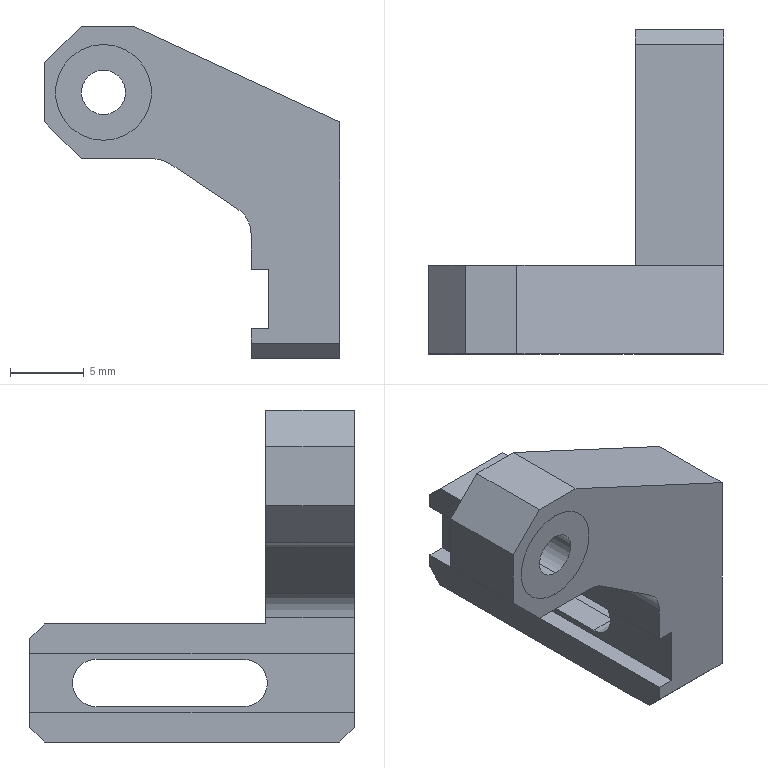Part | SolidWorks | features ICE 10, Chamfer 2, Cut 1, Extrusion 1, Fillet 1 | 2 solids | 43 faces | box 20 x 22 x 22.5 mm | volume 1597 mm3 | plane 29 | cylinder 14 | commonest cylinder face diameters 4 x4 6.5 x4 3 x2 3.2 x2 6 x2
STEP:
#1=CARTESIAN_POINT('',(-6.,-6.,19.5));
#2=VERTEX_POINT('',#1);
#3=CARTESIAN_POINT('',(-6.,-6.,16.5));
#4=VERTEX_POINT('',#3);
#5=CARTESIAN_POINT('',(-6.,-6.,18.));
#6=DIRECTION('',(0.,-1.,0.));
#7=DIRECTION('',(0.,0.,-1.));
#8=AXIS2_PLACEMENT_3D('',#5,#6,#7);
#9=CIRCLE('',#8,1.5);
#10=EDGE_CURVE('',#2,#4,#9,.T.);
#11=ORIENTED_EDGE('',*,*,#10,.F.);
#12=CARTESIAN_POINT('',(-6.,-11.,19.5));
#13=VERTEX_POINT('',#12);
#14=CARTESIAN_POINT('',(-6.,3.192,19.5));
#15=DIRECTION('',(0.,-1.,0.));
#16=VECTOR('',#15,1000.);
#17=LINE('',#14,#16);
#18=EDGE_CURVE('',#2,#13,#17,.T.);
#19=ORIENTED_EDGE('',*,*,#18,.T.);
#20=CARTESIAN_POINT('',(-6.,-11.,16.5));
#21=VERTEX_POINT('',#20);
#22=CARTESIAN_POINT('',(-6.,-11.,18.));
#23=DIRECTION('',(0.,1.,0.));
#24=DIRECTION('',(0.,0.,1.));
#25=AXIS2_PLACEMENT_3D('',#22,#23,#24);
#26=CIRCLE('',#25,1.5);
#27=EDGE_CURVE('',#21,#13,#26,.T.);
#28=ORIENTED_EDGE('',*,*,#27,.F.);
#29=CARTESIAN_POINT('',(-6.,3.192,16.5));
#30=DIRECTION('',(0.,-1.,0.));
#31=VECTOR('',#30,1000.);
#32=LINE('',#29,#31);
#33=EDGE_CURVE('',#4,#21,#32,.T.);
#34=ORIENTED_EDGE('',*,*,#33,.F.);
#35=EDGE_LOOP('',(#11,#19,#28,#34));
#36=FACE_OUTER_BOUND('',#35,.T.);
#37=CARTESIAN_POINT('',(-6.,3.192,18.));
#38=DIRECTION('',(0.,-1.,0.));
#39=DIRECTION('',(0.,0.,-1.));
#40=AXIS2_PLACEMENT_3D('',#37,#38,#39);
#41=CYLINDRICAL_SURFACE('',#40,1.5);
#42=ADVANCED_FACE('',(#36),#41,.F.);
#43=CARTESIAN_POINT('',(-6.,-6.,14.75));
#44=VERTEX_POINT('',#43);
#45=CARTESIAN_POINT('',(-6.,-6.,21.25));
#46=VERTEX_POINT('',#45);
#47=CARTESIAN_POINT('',(-6.,-6.,18.));
#48=DIRECTION('',(0.,-1.,0.));
#49=DIRECTION('',(0.,0.,-1.));
#50=AXIS2_PLACEMENT_3D('',#47,#48,#49);
#51=CIRCLE('',#50,3.25);
#52=EDGE_CURVE('',#44,#46,#51,.T.);
#53=ORIENTED_EDGE('',*,*,#52,.T.);
#54=CARTESIAN_POINT('',(-6.,-11.,21.25));
#55=VERTEX_POINT('',#54);
#56=CARTESIAN_POINT('',(-6.,3.192,21.25));
#57=DIRECTION('',(0.,-1.,0.));
#58=VECTOR('',#57,1000.);
#59=LINE('',#56,#58);
#60=EDGE_CURVE('',#46,#55,#59,.T.);
#61=ORIENTED_EDGE('',*,*,#60,.T.);
#62=CARTESIAN_POINT('',(-6.,-11.,14.75));
#63=VERTEX_POINT('',#62);
#64=CARTESIAN_POINT('',(-6.,-11.,18.));
#65=DIRECTION('',(0.,1.,0.));
#66=DIRECTION('',(0.,0.,1.));
#67=AXIS2_PLACEMENT_3D('',#64,#65,#66);
#68=CIRCLE('',#67,3.25);
#69=EDGE_CURVE('',#55,#63,#68,.T.);
#70=ORIENTED_EDGE('',*,*,#69,.T.);
#71=CARTESIAN_POINT('',(-6.,3.192,14.75));
#72=DIRECTION('',(0.,-1.,0.));
#73=VECTOR('',#72,1000.);
#74=LINE('',#71,#73);
#75=EDGE_CURVE('',#44,#63,#74,.T.);
#76=ORIENTED_EDGE('',*,*,#75,.F.);
#77=EDGE_LOOP('',(#53,#61,#70,#76));
#78=FACE_OUTER_BOUND('',#77,.T.);
#79=CARTESIAN_POINT('',(-6.,3.192,18.));
#80=DIRECTION('',(0.,-1.,0.));
#81=DIRECTION('',(0.,0.,-1.));
#82=AXIS2_PLACEMENT_3D('',#79,#80,#81);
#83=CYLINDRICAL_SURFACE('',#82,3.25);
#84=ADVANCED_FACE('',(#78),#83,.T.);
#85=CARTESIAN_POINT('',(-6.,-11.,18.));
#86=DIRECTION('',(0.,1.,0.));
#87=DIRECTION('',(0.,0.,1.));
#88=AXIS2_PLACEMENT_3D('',#85,#86,#87);
#89=CIRCLE('',#88,3.25);
#90=EDGE_CURVE('',#63,#55,#89,.T.);
#91=ORIENTED_EDGE('',*,*,#90,.F.);
#92=ORIENTED_EDGE('',*,*,#69,.F.);
#93=EDGE_LOOP('',(#91,#92));
#94=FACE_OUTER_BOUND('',#93,.T.);
#95=ORIENTED_EDGE('',*,*,#27,.T.);
#96=CARTESIAN_POINT('',(-6.,-11.,18.));
#97=DIRECTION('',(0.,1.,0.));
#98=DIRECTION('',(0.,0.,1.));
#99=AXIS2_PLACEMENT_3D('',#96,#97,#98);
#100=CIRCLE('',#99,1.5);
#101=EDGE_CURVE('',#13,#21,#100,.T.);
#102=ORIENTED_EDGE('',*,*,#101,.T.);
#103=EDGE_LOOP('',(#95,#102));
#104=FACE_BOUND('',#103,.T.);
#105=CARTESIAN_POINT('',(-6.,-11.,18.));
#106=DIRECTION('',(0.,1.,0.));
#107=DIRECTION('',(0.,0.,1.));
#108=AXIS2_PLACEMENT_3D('',#105,#106,#107);
#109=PLANE('',#108);
#110=ADVANCED_FACE('',(#94,#104),#109,.F.);
#111=ORIENTED_EDGE('',*,*,#60,.F.);
#112=CARTESIAN_POINT('',(-6.,-6.,18.));
#113=DIRECTION('',(0.,-1.,0.));
#114=DIRECTION('',(0.,0.,-1.));
#115=AXIS2_PLACEMENT_3D('',#112,#113,#114);
#116=CIRCLE('',#115,3.25);
#117=EDGE_CURVE('',#46,#44,#116,.T.);
#118=ORIENTED_EDGE('',*,*,#117,.T.);
#119=ORIENTED_EDGE('',*,*,#75,.T.);
#120=ORIENTED_EDGE('',*,*,#90,.T.);
#121=EDGE_LOOP('',(#111,#118,#119,#120));
#122=FACE_OUTER_BOUND('',#121,.T.);
#123=CARTESIAN_POINT('',(-6.,3.192,18.));
#124=DIRECTION('',(0.,-1.,0.));
#125=DIRECTION('',(0.,0.,-1.));
#126=AXIS2_PLACEMENT_3D('',#123,#124,#125);
#127=CYLINDRICAL_SURFACE('',#126,3.25);
#128=ADVANCED_FACE('',(#122),#127,.T.);
#129=ORIENTED_EDGE('',*,*,#18,.F.);
#130=CARTESIAN_POINT('',(-6.,-6.,18.));
#131=DIRECTION('',(0.,-1.,0.));
#132=DIRECTION('',(0.,0.,-1.));
#133=AXIS2_PLACEMENT_3D('',#130,#131,#132);
#134=CIRCLE('',#133,1.5);
#135=EDGE_CURVE('',#4,#2,#134,.T.);
#136=ORIENTED_EDGE('',*,*,#135,.F.);
#137=ORIENTED_EDGE('',*,*,#33,.T.);
#138=ORIENTED_EDGE('',*,*,#101,.F.);
#139=EDGE_LOOP('',(#129,#136,#137,#138));
#140=FACE_OUTER_BOUND('',#139,.T.);
#141=CARTESIAN_POINT('',(-6.,3.192,18.));
#142=DIRECTION('',(0.,-1.,0.));
#143=DIRECTION('',(0.,0.,-1.));
#144=AXIS2_PLACEMENT_3D('',#141,#142,#143);
#145=CYLINDRICAL_SURFACE('',#144,1.5);
#146=ADVANCED_FACE('',(#140),#145,.F.);
#147=ORIENTED_EDGE('',*,*,#52,.F.);
#148=ORIENTED_EDGE('',*,*,#117,.F.);
#149=EDGE_LOOP('',(#147,#148));
#150=FACE_OUTER_BOUND('',#149,.T.);
#151=ORIENTED_EDGE('',*,*,#135,.T.);
#152=ORIENTED_EDGE('',*,*,#10,.T.);
#153=EDGE_LOOP('',(#151,#152));
#154=FACE_BOUND('',#153,.T.);
#155=CARTESIAN_POINT('',(-10.,-6.,22.5));
#156=DIRECTION('',(0.,-1.,0.));
#157=DIRECTION('',(0.,0.,-1.));
#158=AXIS2_PLACEMENT_3D('',#155,#156,#157);
#159=PLANE('',#158);
#160=ADVANCED_FACE('',(#150,#154),#159,.F.);
#161=CLOSED_SHELL('',(#42,#84,#110,#128,#146,#160));
#162=MANIFOLD_SOLID_BREP('',#161);
#163=CARTESIAN_POINT('',(-6.,-6.,16.));
#164=VERTEX_POINT('',#163);
#165=CARTESIAN_POINT('',(-6.,-6.,20.));
#166=VERTEX_POINT('',#165);
#167=CARTESIAN_POINT('',(-6.,-6.,18.));
#168=DIRECTION('',(0.,1.,0.));
#169=DIRECTION('',(0.,0.,1.));
#170=AXIS2_PLACEMENT_3D('',#167,#168,#169);
#171=CIRCLE('',#170,2.);
#172=EDGE_CURVE('',#164,#166,#171,.T.);
#173=ORIENTED_EDGE('',*,*,#172,.F.);
#174=CARTESIAN_POINT('',(-6.,-5.,16.));
#175=VERTEX_POINT('',#174);
#176=CARTESIAN_POINT('',(-6.,-6.,16.));
#177=DIRECTION('',(0.,1.,0.));
#178=VECTOR('',#177,1000.);
#179=LINE('',#176,#178);
#180=EDGE_CURVE('',#164,#175,#179,.T.);
#181=ORIENTED_EDGE('',*,*,#180,.T.);
#182=CARTESIAN_POINT('',(-6.,-5.,20.));
#183=VERTEX_POINT('',#182);
#184=CARTESIAN_POINT('',(-6.,-5.,18.));
#185=DIRECTION('',(0.,1.,0.));
#186=DIRECTION('',(0.,0.,1.));
#187=AXIS2_PLACEMENT_3D('',#184,#185,#186);
#188=CIRCLE('',#187,2.);
#189=EDGE_CURVE('',#175,#183,#188,.T.);
#190=ORIENTED_EDGE('',*,*,#189,.T.);
#191=CARTESIAN_POINT('',(-6.,-6.,20.));
#192=DIRECTION('',(0.,1.,0.));
#193=VECTOR('',#192,1000.);
#194=LINE('',#191,#193);
#195=EDGE_CURVE('',#166,#183,#194,.T.);
#196=ORIENTED_EDGE('',*,*,#195,.F.);
#197=EDGE_LOOP('',(#173,#181,#190,#196));
#198=FACE_OUTER_BOUND('',#197,.T.);
#199=CARTESIAN_POINT('',(-6.,-6.,18.));
#200=DIRECTION('',(0.,1.,0.));
#201=DIRECTION('',(0.,0.,1.));
#202=AXIS2_PLACEMENT_3D('',#199,#200,#201);
#203=CYLINDRICAL_SURFACE('',#202,2.);
#204=ADVANCED_FACE('',(#198),#203,.F.);
#205=CARTESIAN_POINT('',(-6.,-6.,21.25));
#206=VERTEX_POINT('',#205);
#207=CARTESIAN_POINT('',(-6.,-6.,14.75));
#208=VERTEX_POINT('',#207);
#209=CARTESIAN_POINT('',(-6.,-6.,18.));
#210=DIRECTION('',(0.,-1.,0.));
#211=DIRECTION('',(0.,0.,-1.));
#212=AXIS2_PLACEMENT_3D('',#209,#210,#211);
#213=CIRCLE('',#212,3.25);
#214=EDGE_CURVE('',#206,#208,#213,.T.);
#215=ORIENTED_EDGE('',*,*,#214,.F.);
#216=CARTESIAN_POINT('',(-6.,-11.,21.25));
#217=VERTEX_POINT('',#216);
#218=CARTESIAN_POINT('',(-6.,4.192,21.25));
#219=DIRECTION('',(0.,-1.,0.));
#220=VECTOR('',#219,1000.);
#221=LINE('',#218,#220);
#222=EDGE_CURVE('',#206,#217,#221,.T.);
#223=ORIENTED_EDGE('',*,*,#222,.T.);
#224=CARTESIAN_POINT('',(-6.,-11.,14.75));
#225=VERTEX_POINT('',#224);
#226=CARTESIAN_POINT('',(-6.,-11.,18.));
#227=DIRECTION('',(0.,1.,0.));
#228=DIRECTION('',(0.,0.,1.));
#229=AXIS2_PLACEMENT_3D('',#226,#227,#228);
#230=CIRCLE('',#229,3.25);
#231=EDGE_CURVE('',#225,#217,#230,.T.);
#232=ORIENTED_EDGE('',*,*,#231,.F.);
#233=CARTESIAN_POINT('',(-6.,4.192,14.75));
#234=DIRECTION('',(0.,-1.,0.));
#235=VECTOR('',#234,1000.);
#236=LINE('',#233,#235);
#237=EDGE_CURVE('',#208,#225,#236,.T.);
#238=ORIENTED_EDGE('',*,*,#237,.F.);
#239=EDGE_LOOP('',(#215,#223,#232,#238));
#240=FACE_OUTER_BOUND('',#239,.T.);
#241=CARTESIAN_POINT('',(-6.,4.192,18.));
#242=DIRECTION('',(0.,-1.,0.));
#243=DIRECTION('',(0.,0.,-1.));
#244=AXIS2_PLACEMENT_3D('',#241,#242,#243);
#245=CYLINDRICAL_SURFACE('',#244,3.25);
#246=ADVANCED_FACE('',(#240),#245,.F.);
#247=CARTESIAN_POINT('',(7.,-3.5,2.4));
#248=VERTEX_POINT('',#247);
#249=CARTESIAN_POINT('',(7.,-3.5,5.6));
#250=VERTEX_POINT('',#249);
#251=CARTESIAN_POINT('',(7.,-3.5,4.));
#252=DIRECTION('',(-1.,0.,0.));
#253=DIRECTION('',(0.,0.,-1.));
#254=AXIS2_PLACEMENT_3D('',#251,#252,#253);
#255=CIRCLE('',#254,1.6);
#256=EDGE_CURVE('',#248,#250,#255,.T.);
#257=ORIENTED_EDGE('',*,*,#256,.F.);
#258=CARTESIAN_POINT('',(5.2,-3.5,2.4));
#259=VERTEX_POINT('',#258);
#260=CARTESIAN_POINT('',(-10.,-3.5,2.4));
#261=DIRECTION('',(1.,0.,0.));
#262=VECTOR('',#261,1000.);
#263=LINE('',#260,#262);
#264=EDGE_CURVE('',#259,#248,#263,.T.);
#265=ORIENTED_EDGE('',*,*,#264,.F.);
#266=CARTESIAN_POINT('',(5.2,-3.5,5.6));
#267=VERTEX_POINT('',#266);
#268=CARTESIAN_POINT('',(5.2,-3.5,4.));
#269=DIRECTION('',(-1.,0.,0.));
#270=DIRECTION('',(0.,0.,1.));
#271=AXIS2_PLACEMENT_3D('',#268,#269,#270);
#272=CIRCLE('',#271,1.6);
#273=EDGE_CURVE('',#259,#267,#272,.T.);
#274=ORIENTED_EDGE('',*,*,#273,.T.);
#275=CARTESIAN_POINT('',(-10.,-3.5,5.6));
#276=DIRECTION('',(1.,0.,0.));
#277=VECTOR('',#276,1000.);
#278=LINE('',#275,#277);
#279=EDGE_CURVE('',#267,#250,#278,.T.);
#280=ORIENTED_EDGE('',*,*,#279,.T.);
#281=EDGE_LOOP('',(#257,#265,#274,#280));
#282=FACE_OUTER_BOUND('',#281,.T.);
#283=CARTESIAN_POINT('',(-10.,-3.5,4.));
#284=DIRECTION('',(1.,0.,0.));
#285=DIRECTION('',(0.,0.,-1.));
#286=AXIS2_PLACEMENT_3D('',#283,#284,#285);
#287=CYLINDRICAL_SURFACE('',#286,1.6);
#288=ADVANCED_FACE('',(#282),#287,.F.);
#289=CARTESIAN_POINT('',(7.,6.5,5.6));
#290=VERTEX_POINT('',#289);
#291=CARTESIAN_POINT('',(7.,-3.5,5.6));
#292=DIRECTION('',(0.,1.,0.));
#293=VECTOR('',#292,1000.);
#294=LINE('',#291,#293);
#295=EDGE_CURVE('',#250,#290,#294,.T.);
#296=ORIENTED_EDGE('',*,*,#295,.F.);
#297=ORIENTED_EDGE('',*,*,#279,.F.);
#298=CARTESIAN_POINT('',(5.2,6.5,5.6));
#299=VERTEX_POINT('',#298);
#300=CARTESIAN_POINT('',(5.2,0.,5.6));
#301=DIRECTION('',(0.,1.,0.));
#302=VECTOR('',#301,1000.);
#303=LINE('',#300,#302);
#304=EDGE_CURVE('',#267,#299,#303,.T.);
#305=ORIENTED_EDGE('',*,*,#304,.T.);
#306=CARTESIAN_POINT('',(-10.,6.5,5.6));
#307=DIRECTION('',(1.,0.,0.));
#308=VECTOR('',#307,1000.);
#309=LINE('',#306,#308);
#310=EDGE_CURVE('',#299,#290,#309,.T.);
#311=ORIENTED_EDGE('',*,*,#310,.T.);
#312=EDGE_LOOP('',(#296,#297,#305,#311));
#313=FACE_OUTER_BOUND('',#312,.T.);
#314=CARTESIAN_POINT('',(-10.,-3.5,5.6));
#315=DIRECTION('',(0.,0.,1.));
#316=DIRECTION('',(1.,0.,0.));
#317=AXIS2_PLACEMENT_3D('',#314,#315,#316);
#318=PLANE('',#317);
#319=ADVANCED_FACE('',(#313),#318,.F.);
#320=CARTESIAN_POINT('',(7.,6.5,2.4));
#321=VERTEX_POINT('',#320);
#322=CARTESIAN_POINT('',(7.,6.5,4.));
#323=DIRECTION('',(-1.,0.,0.));
#324=DIRECTION('',(0.,0.,-1.));
#325=AXIS2_PLACEMENT_3D('',#322,#323,#324);
#326=CIRCLE('',#325,1.6);
#327=EDGE_CURVE('',#290,#321,#326,.T.);
#328=ORIENTED_EDGE('',*,*,#327,.F.);
#329=ORIENTED_EDGE('',*,*,#310,.F.);
#330=CARTESIAN_POINT('',(5.2,6.5,2.4));
#331=VERTEX_POINT('',#330);
#332=CARTESIAN_POINT('',(5.2,6.5,4.));
#333=DIRECTION('',(-1.,0.,0.));
#334=DIRECTION('',(0.,0.,1.));
#335=AXIS2_PLACEMENT_3D('',#332,#333,#334);
#336=CIRCLE('',#335,1.6);
#337=EDGE_CURVE('',#299,#331,#336,.T.);
#338=ORIENTED_EDGE('',*,*,#337,.T.);
#339=CARTESIAN_POINT('',(-10.,6.5,2.4));
#340=DIRECTION('',(1.,0.,0.));
#341=VECTOR('',#340,1000.);
#342=LINE('',#339,#341);
#343=EDGE_CURVE('',#331,#321,#342,.T.);
#344=ORIENTED_EDGE('',*,*,#343,.T.);
#345=EDGE_LOOP('',(#328,#329,#338,#344));
#346=FACE_OUTER_BOUND('',#345,.T.);
#347=CARTESIAN_POINT('',(-10.,6.5,4.));
#348=DIRECTION('',(1.,0.,0.));
#349=DIRECTION('',(0.,0.,-1.));
#350=AXIS2_PLACEMENT_3D('',#347,#348,#349);
#351=CYLINDRICAL_SURFACE('',#350,1.6);
#352=ADVANCED_FACE('',(#346),#351,.F.);
#353=CARTESIAN_POINT('',(7.,-3.5,2.4));
#354=DIRECTION('',(0.,-1.,0.));
#355=VECTOR('',#354,1000.);
#356=LINE('',#353,#355);
#357=EDGE_CURVE('',#321,#248,#356,.T.);
#358=ORIENTED_EDGE('',*,*,#357,.F.);
#359=ORIENTED_EDGE('',*,*,#343,.F.);
#360=CARTESIAN_POINT('',(5.2,0.,2.4));
#361=DIRECTION('',(0.,-1.,0.));
#362=VECTOR('',#361,1000.);
#363=LINE('',#360,#362);
#364=EDGE_CURVE('',#331,#259,#363,.T.);
#365=ORIENTED_EDGE('',*,*,#364,.T.);
#366=ORIENTED_EDGE('',*,*,#264,.T.);
#367=EDGE_LOOP('',(#358,#359,#365,#366));
#368=FACE_OUTER_BOUND('',#367,.T.);
#369=CARTESIAN_POINT('',(-10.,-3.5,2.4));
#370=DIRECTION('',(0.,0.,-1.));
#371=DIRECTION('',(-1.,0.,0.));
#372=AXIS2_PLACEMENT_3D('',#369,#370,#371);
#373=PLANE('',#372);
#374=ADVANCED_FACE('',(#368),#373,.F.);
#375=CARTESIAN_POINT('',(4.,-11.,6.));
#376=VERTEX_POINT('',#375);
#377=CARTESIAN_POINT('',(4.,-11.,8.43));
#378=VERTEX_POINT('',#377);
#379=CARTESIAN_POINT('',(4.,-11.,0.));
#380=DIRECTION('',(0.,0.,1.));
#381=VECTOR('',#380,1000.);
#382=LINE('',#379,#381);
#383=EDGE_CURVE('',#376,#378,#382,.T.);
#384=ORIENTED_EDGE('',*,*,#383,.T.);
#385=CARTESIAN_POINT('',(4.,-5.,8.43));
#386=VERTEX_POINT('',#385);
#387=CARTESIAN_POINT('',(4.,11.,8.43));
#388=DIRECTION('',(0.,1.,0.));
#389=VECTOR('',#388,1000.);
#390=LINE('',#387,#389);
#391=EDGE_CURVE('',#378,#386,#390,.T.);
#392=ORIENTED_EDGE('',*,*,#391,.T.);
#393=CARTESIAN_POINT('',(4.,-5.,8.));
#394=VERTEX_POINT('',#393);
#395=CARTESIAN_POINT('',(4.,-5.,22.5));
#396=DIRECTION('',(0.,0.,1.));
#397=VECTOR('',#396,1000.);
#398=LINE('',#395,#397);
#399=EDGE_CURVE('',#394,#386,#398,.T.);
#400=ORIENTED_EDGE('',*,*,#399,.F.);
#401=CARTESIAN_POINT('',(4.,10.,8.));
#402=VERTEX_POINT('',#401);
#403=CARTESIAN_POINT('',(4.,0.,8.));
#404=DIRECTION('',(0.,-1.,0.));
#405=VECTOR('',#404,1000.);
#406=LINE('',#403,#405);
#407=EDGE_CURVE('',#402,#394,#406,.T.);
#408=ORIENTED_EDGE('',*,*,#407,.F.);
#409=CARTESIAN_POINT('',(4.,11.,7.));
#410=VERTEX_POINT('',#409);
#411=CARTESIAN_POINT('',(4.,10.,8.));
#412=DIRECTION('',(0.,0.7071,-0.7071));
#413=VECTOR('',#412,1000.);
#414=LINE('',#411,#413);
#415=EDGE_CURVE('',#402,#410,#414,.T.);
#416=ORIENTED_EDGE('',*,*,#415,.T.);
#417=CARTESIAN_POINT('',(4.,11.,6.));
#418=VERTEX_POINT('',#417);
#419=CARTESIAN_POINT('',(4.,11.,8.));
#420=DIRECTION('',(0.,0.,1.));
#421=VECTOR('',#420,1000.);
#422=LINE('',#419,#421);
#423=EDGE_CURVE('',#418,#410,#422,.T.);
#424=ORIENTED_EDGE('',*,*,#423,.F.);
#425=CARTESIAN_POINT('',(4.,-11.,6.));
#426=DIRECTION('',(0.,1.,0.));
#427=VECTOR('',#426,1000.);
#428=LINE('',#425,#427);
#429=EDGE_CURVE('',#376,#418,#428,.T.);
#430=ORIENTED_EDGE('',*,*,#429,.F.);
#431=EDGE_LOOP('',(#384,#392,#400,#408,#416,#424,#430));
#432=FACE_OUTER_BOUND('',#431,.T.);
#433=CARTESIAN_POINT('',(4.,11.,0.));
#434=DIRECTION('',(1.,0.,0.));
#435=DIRECTION('',(0.,0.,-1.));
#436=AXIS2_PLACEMENT_3D('',#433,#434,#435);
#437=PLANE('',#436);
#438=ADVANCED_FACE('',(#432),#437,.F.);
#439=CARTESIAN_POINT('',(4.,-11.,1.));
#440=VERTEX_POINT('',#439);
#441=CARTESIAN_POINT('',(4.,-11.,2.));
#442=VERTEX_POINT('',#441);
#443=CARTESIAN_POINT('',(4.,-11.,0.));
#444=DIRECTION('',(0.,0.,1.));
#445=VECTOR('',#444,1000.);
#446=LINE('',#443,#445);
#447=EDGE_CURVE('',#440,#442,#446,.T.);
#448=ORIENTED_EDGE('',*,*,#447,.F.);
#449=CARTESIAN_POINT('',(10.,-11.,1.));
#450=VERTEX_POINT('',#449);
#451=CARTESIAN_POINT('',(10.,-11.,1.));
#452=DIRECTION('',(1.,0.,0.));
#453=VECTOR('',#452,1000.);
#454=LINE('',#451,#453);
#455=EDGE_CURVE('',#440,#450,#454,.T.);
#456=ORIENTED_EDGE('',*,*,#455,.T.);
#457=CARTESIAN_POINT('',(10.,-11.,16.));
#458=VERTEX_POINT('',#457);
#459=CARTESIAN_POINT('',(10.,-11.,8.));
#460=DIRECTION('',(0.,0.,-1.));
#461=VECTOR('',#460,1000.);
#462=LINE('',#459,#461);
#463=EDGE_CURVE('',#458,#450,#462,.T.);
#464=ORIENTED_EDGE('',*,*,#463,.F.);
#465=CARTESIAN_POINT('',(-4.,-11.,22.5));
#466=VERTEX_POINT('',#465);
#467=CARTESIAN_POINT('',(-4.,-11.,22.5));
#468=DIRECTION('',(0.907,0.,-0.4211));
#469=VECTOR('',#468,1000.);
#470=LINE('',#467,#469);
#471=EDGE_CURVE('',#466,#458,#470,.T.);
#472=ORIENTED_EDGE('',*,*,#471,.F.);
#473=CARTESIAN_POINT('',(-7.5,-11.,22.5));
#474=VERTEX_POINT('',#473);
#475=CARTESIAN_POINT('',(-10.,-11.,22.5));
#476=DIRECTION('',(1.,0.,0.));
#477=VECTOR('',#476,1000.);
#478=LINE('',#475,#477);
#479=EDGE_CURVE('',#474,#466,#478,.T.);
#480=ORIENTED_EDGE('',*,*,#479,.F.);
#481=CARTESIAN_POINT('',(-10.,-11.,20.));
#482=VERTEX_POINT('',#481);
#483=CARTESIAN_POINT('',(-7.5,-11.,22.5));
#484=DIRECTION('',(-0.7071,0.,-0.7071));
#485=VECTOR('',#484,1000.);
#486=LINE('',#483,#485);
#487=EDGE_CURVE('',#474,#482,#486,.T.);
#488=ORIENTED_EDGE('',*,*,#487,.T.);
#489=CARTESIAN_POINT('',(-10.,-11.,16.));
#490=VERTEX_POINT('',#489);
#491=CARTESIAN_POINT('',(-10.,-11.,8.));
#492=DIRECTION('',(0.,0.,-1.));
#493=VECTOR('',#492,1000.);
#494=LINE('',#491,#493);
#495=EDGE_CURVE('',#482,#490,#494,.T.);
#496=ORIENTED_EDGE('',*,*,#495,.T.);
#497=CARTESIAN_POINT('',(-7.5,-11.,13.5));
#498=VERTEX_POINT('',#497);
#499=CARTESIAN_POINT('',(-10.,-11.,16.));
#500=DIRECTION('',(0.7071,0.,-0.7071));
#501=VECTOR('',#500,1000.);
#502=LINE('',#499,#501);
#503=EDGE_CURVE('',#490,#498,#502,.T.);
#504=ORIENTED_EDGE('',*,*,#503,.T.);
#505=CARTESIAN_POINT('',(-2.606,-11.,13.5));
#506=VERTEX_POINT('',#505);
#507=CARTESIAN_POINT('',(4.,-11.,13.5));
#508=DIRECTION('',(-1.,0.,0.));
#509=VECTOR('',#508,1000.);
#510=LINE('',#507,#509);
#511=EDGE_CURVE('',#506,#498,#510,.T.);
#512=ORIENTED_EDGE('',*,*,#511,.F.);
#513=CARTESIAN_POINT('',(-1.496,-11.,13.164));
#514=VERTEX_POINT('',#513);
#515=CARTESIAN_POINT('',(-2.606,-11.,11.5));
#516=DIRECTION('',(0.,1.,0.));
#517=DIRECTION('',(0.,0.,1.));
#518=AXIS2_PLACEMENT_3D('',#515,#516,#517);
#519=CIRCLE('',#518,2.);
#520=EDGE_CURVE('',#506,#514,#519,.T.);
#521=ORIENTED_EDGE('',*,*,#520,.T.);
#522=CARTESIAN_POINT('',(3.109,-11.,10.094));
#523=VERTEX_POINT('',#522);
#524=CARTESIAN_POINT('',(-2.,-11.,13.5));
#525=DIRECTION('',(0.8321,0.,-0.5547));
#526=VECTOR('',#525,1000.);
#527=LINE('',#524,#526);
#528=EDGE_CURVE('',#514,#523,#527,.T.);
#529=ORIENTED_EDGE('',*,*,#528,.T.);
#530=CARTESIAN_POINT('',(2.,-11.,8.43));
#531=DIRECTION('',(0.,1.,0.));
#532=DIRECTION('',(0.,0.,1.));
#533=AXIS2_PLACEMENT_3D('',#530,#531,#532);
#534=CIRCLE('',#533,2.);
#535=EDGE_CURVE('',#523,#378,#534,.T.);
#536=ORIENTED_EDGE('',*,*,#535,.T.);
#537=ORIENTED_EDGE('',*,*,#383,.F.);
#538=CARTESIAN_POINT('',(5.2,-11.,6.));
#539=VERTEX_POINT('',#538);
#540=CARTESIAN_POINT('',(5.2,-11.,6.));
#541=DIRECTION('',(-1.,0.,0.));
#542=VECTOR('',#541,1000.);
#543=LINE('',#540,#542);
#544=EDGE_CURVE('',#539,#376,#543,.T.);
#545=ORIENTED_EDGE('',*,*,#544,.F.);
#546=CARTESIAN_POINT('',(5.2,-11.,2.));
#547=VERTEX_POINT('',#546);
#548=CARTESIAN_POINT('',(5.2,-11.,6.));
#549=DIRECTION('',(0.,0.,1.));
#550=VECTOR('',#549,1000.);
#551=LINE('',#548,#550);
#552=EDGE_CURVE('',#547,#539,#551,.T.);
#553=ORIENTED_EDGE('',*,*,#552,.F.);
#554=CARTESIAN_POINT('',(5.2,-11.,2.));
#555=DIRECTION('',(-1.,0.,0.));
#556=VECTOR('',#555,1000.);
#557=LINE('',#554,#556);
#558=EDGE_CURVE('',#547,#442,#557,.T.);
#559=ORIENTED_EDGE('',*,*,#558,.T.);
#560=EDGE_LOOP('',(#448,#456,#464,#472,#480,#488,#496,#504,#512,#521,#529,#536,#537,#545,#553,#559));
#561=FACE_OUTER_BOUND('',#560,.T.);
#562=ORIENTED_EDGE('',*,*,#231,.T.);
#563=CARTESIAN_POINT('',(-6.,-11.,18.));
#564=DIRECTION('',(0.,1.,0.));
#565=DIRECTION('',(0.,0.,1.));
#566=AXIS2_PLACEMENT_3D('',#563,#564,#565);
#567=CIRCLE('',#566,3.25);
#568=EDGE_CURVE('',#217,#225,#567,.T.);
#569=ORIENTED_EDGE('',*,*,#568,.T.);
#570=EDGE_LOOP('',(#562,#569));
#571=FACE_BOUND('',#570,.T.);
#572=CARTESIAN_POINT('',(-10.,-11.,8.));
#573=DIRECTION('',(0.,1.,0.));
#574=DIRECTION('',(0.,0.,1.));
#575=AXIS2_PLACEMENT_3D('',#572,#573,#574);
#576=PLANE('',#575);
#577=ADVANCED_FACE('',(#561,#571),#576,.F.);
#578=CARTESIAN_POINT('',(10.,-5.,8.));
#579=VERTEX_POINT('',#578);
#580=CARTESIAN_POINT('',(10.,10.,8.));
#581=VERTEX_POINT('',#580);
#582=CARTESIAN_POINT('',(10.,-11.,8.));
#583=DIRECTION('',(0.,1.,0.));
#584=VECTOR('',#583,1000.);
#585=LINE('',#582,#584);
#586=EDGE_CURVE('',#579,#581,#585,.T.);
#587=ORIENTED_EDGE('',*,*,#586,.T.);
#588=CARTESIAN_POINT('',(0.,10.,8.));
#589=DIRECTION('',(-1.,0.,0.));
#590=VECTOR('',#589,1000.);
#591=LINE('',#588,#590);
#592=EDGE_CURVE('',#581,#402,#591,.T.);
#593=ORIENTED_EDGE('',*,*,#592,.T.);
#594=ORIENTED_EDGE('',*,*,#407,.T.);
#595=CARTESIAN_POINT('',(-10.,-5.,8.));
#596=DIRECTION('',(-1.,0.,0.));
#597=VECTOR('',#596,1000.);
#598=LINE('',#595,#597);
#599=EDGE_CURVE('',#579,#394,#598,.T.);
#600=ORIENTED_EDGE('',*,*,#599,.F.);
#601=EDGE_LOOP('',(#587,#593,#594,#600));
#602=FACE_OUTER_BOUND('',#601,.T.);
#603=CARTESIAN_POINT('',(0.,0.,8.));
#604=DIRECTION('',(0.,0.,-1.));
#605=DIRECTION('',(-1.,0.,0.));
#606=AXIS2_PLACEMENT_3D('',#603,#604,#605);
#607=PLANE('',#606);
#608=ADVANCED_FACE('',(#602),#607,.F.);
#609=CARTESIAN_POINT('',(10.,-3.5,1.));
#610=VERTEX_POINT('',#609);
#611=CARTESIAN_POINT('',(10.,6.5,1.));
#612=VERTEX_POINT('',#611);
#613=CARTESIAN_POINT('',(10.,-3.5,1.));
#614=DIRECTION('',(0.,1.,0.));
#615=VECTOR('',#614,1000.);
#616=LINE('',#613,#615);
#617=EDGE_CURVE('',#610,#612,#616,.T.);
#618=ORIENTED_EDGE('',*,*,#617,.F.);
#619=CARTESIAN_POINT('',(10.,-3.5,7.));
#620=VERTEX_POINT('',#619);
#621=CARTESIAN_POINT('',(10.,-3.5,4.));
#622=DIRECTION('',(1.,0.,0.));
#623=DIRECTION('',(0.,0.,-1.));
#624=AXIS2_PLACEMENT_3D('',#621,#622,#623);
#625=CIRCLE('',#624,3.);
#626=EDGE_CURVE('',#620,#610,#625,.T.);
#627=ORIENTED_EDGE('',*,*,#626,.F.);
#628=CARTESIAN_POINT('',(10.,6.5,7.));
#629=VERTEX_POINT('',#628);
#630=CARTESIAN_POINT('',(10.,-3.5,7.));
#631=DIRECTION('',(0.,-1.,0.));
#632=VECTOR('',#631,1000.);
#633=LINE('',#630,#632);
#634=EDGE_CURVE('',#629,#620,#633,.T.);
#635=ORIENTED_EDGE('',*,*,#634,.F.);
#636=CARTESIAN_POINT('',(10.,6.5,4.));
#637=DIRECTION('',(1.,0.,0.));
#638=DIRECTION('',(0.,0.,-1.));
#639=AXIS2_PLACEMENT_3D('',#636,#637,#638);
#640=CIRCLE('',#639,3.);
#641=EDGE_CURVE('',#612,#629,#640,.T.);
#642=ORIENTED_EDGE('',*,*,#641,.F.);
#643=EDGE_LOOP('',(#618,#627,#635,#642));
#644=FACE_BOUND('',#643,.T.);
#645=ORIENTED_EDGE('',*,*,#463,.T.);
#646=CARTESIAN_POINT('',(10.,-10.,0.));
#647=VERTEX_POINT('',#646);
#648=CARTESIAN_POINT('',(10.,-11.,1.));
#649=DIRECTION('',(0.,0.7071,-0.7071));
#650=VECTOR('',#649,1000.);
#651=LINE('',#648,#650);
#652=EDGE_CURVE('',#450,#647,#651,.T.);
#653=ORIENTED_EDGE('',*,*,#652,.T.);
#654=CARTESIAN_POINT('',(10.,10.,0.));
#655=VERTEX_POINT('',#654);
#656=CARTESIAN_POINT('',(10.,-11.,0.));
#657=DIRECTION('',(0.,1.,0.));
#658=VECTOR('',#657,1000.);
#659=LINE('',#656,#658);
#660=EDGE_CURVE('',#647,#655,#659,.T.);
#661=ORIENTED_EDGE('',*,*,#660,.T.);
#662=CARTESIAN_POINT('',(10.,11.,1.));
#663=VERTEX_POINT('',#662);
#664=CARTESIAN_POINT('',(10.,11.,1.));
#665=DIRECTION('',(0.,0.7071,0.7071));
#666=VECTOR('',#665,1000.);
#667=LINE('',#664,#666);
#668=EDGE_CURVE('',#655,#663,#667,.T.);
#669=ORIENTED_EDGE('',*,*,#668,.T.);
#670=CARTESIAN_POINT('',(10.,11.,7.));
#671=VERTEX_POINT('',#670);
#672=CARTESIAN_POINT('',(10.,11.,8.));
#673=DIRECTION('',(0.,0.,-1.));
#674=VECTOR('',#673,1000.);
#675=LINE('',#672,#674);
#676=EDGE_CURVE('',#671,#663,#675,.T.);
#677=ORIENTED_EDGE('',*,*,#676,.F.);
#678=CARTESIAN_POINT('',(10.,10.,8.));
#679=DIRECTION('',(0.,-0.7071,0.7071));
#680=VECTOR('',#679,1000.);
#681=LINE('',#678,#680);
#682=EDGE_CURVE('',#671,#581,#681,.T.);
#683=ORIENTED_EDGE('',*,*,#682,.T.);
#684=ORIENTED_EDGE('',*,*,#586,.F.);
#685=CARTESIAN_POINT('',(10.,-5.,16.));
#686=VERTEX_POINT('',#685);
#687=CARTESIAN_POINT('',(10.,-5.,22.5));
#688=DIRECTION('',(0.,0.,-1.));
#689=VECTOR('',#688,1000.);
#690=LINE('',#687,#689);
#691=EDGE_CURVE('',#686,#579,#690,.T.);
#692=ORIENTED_EDGE('',*,*,#691,.F.);
#693=CARTESIAN_POINT('',(10.,11.,16.));
#694=DIRECTION('',(0.,-1.,0.));
#695=VECTOR('',#694,1000.);
#696=LINE('',#693,#695);
#697=EDGE_CURVE('',#686,#458,#696,.T.);
#698=ORIENTED_EDGE('',*,*,#697,.T.);
#699=EDGE_LOOP('',(#645,#653,#661,#669,#677,#683,#684,#692,#698));
#700=FACE_OUTER_BOUND('',#699,.T.);
#701=CARTESIAN_POINT('',(10.,-11.,8.));
#702=DIRECTION('',(-1.,0.,0.));
#703=DIRECTION('',(0.,0.,1.));
#704=AXIS2_PLACEMENT_3D('',#701,#702,#703);
#705=PLANE('',#704);
#706=ADVANCED_FACE('',(#644,#700),#705,.F.);
#707=ORIENTED_EDGE('',*,*,#423,.T.);
#708=CARTESIAN_POINT('',(-10.,11.,7.));
#709=DIRECTION('',(1.,0.,0.));
#710=VECTOR('',#709,1000.);
#711=LINE('',#708,#710);
#712=EDGE_CURVE('',#410,#671,#711,.T.);
#713=ORIENTED_EDGE('',*,*,#712,.T.);
#714=ORIENTED_EDGE('',*,*,#676,.T.);
#715=CARTESIAN_POINT('',(4.,11.,1.));
#716=VERTEX_POINT('',#715);
#717=CARTESIAN_POINT('',(4.,11.,1.));
#718=DIRECTION('',(-1.,0.,0.));
#719=VECTOR('',#718,1000.);
#720=LINE('',#717,#719);
#721=EDGE_CURVE('',#663,#716,#720,.T.);
#722=ORIENTED_EDGE('',*,*,#721,.T.);
#723=CARTESIAN_POINT('',(4.,11.,2.));
#724=VERTEX_POINT('',#723);
#725=CARTESIAN_POINT('',(4.,11.,8.));
#726=DIRECTION('',(0.,0.,1.));
#727=VECTOR('',#726,1000.);
#728=LINE('',#725,#727);
#729=EDGE_CURVE('',#716,#724,#728,.T.);
#730=ORIENTED_EDGE('',*,*,#729,.T.);
#731=CARTESIAN_POINT('',(5.2,11.,2.));
#732=VERTEX_POINT('',#731);
#733=CARTESIAN_POINT('',(5.2,11.,2.));
#734=DIRECTION('',(-1.,0.,0.));
#735=VECTOR('',#734,1000.);
#736=LINE('',#733,#735);
#737=EDGE_CURVE('',#732,#724,#736,.T.);
#738=ORIENTED_EDGE('',*,*,#737,.F.);
#739=CARTESIAN_POINT('',(5.2,11.,6.));
#740=VERTEX_POINT('',#739);
#741=CARTESIAN_POINT('',(5.2,11.,6.));
#742=DIRECTION('',(0.,0.,-1.));
#743=VECTOR('',#742,1000.);
#744=LINE('',#741,#743);
#745=EDGE_CURVE('',#740,#732,#744,.T.);
#746=ORIENTED_EDGE('',*,*,#745,.F.);
#747=CARTESIAN_POINT('',(5.2,11.,6.));
#748=DIRECTION('',(-1.,0.,0.));
#749=VECTOR('',#748,1000.);
#750=LINE('',#747,#749);
#751=EDGE_CURVE('',#740,#418,#750,.T.);
#752=ORIENTED_EDGE('',*,*,#751,.T.);
#753=EDGE_LOOP('',(#707,#713,#714,#722,#730,#738,#746,#752));
#754=FACE_OUTER_BOUND('',#753,.T.);
#755=CARTESIAN_POINT('',(-10.,11.,8.));
#756=DIRECTION('',(0.,-1.,0.));
#757=DIRECTION('',(0.,0.,-1.));
#758=AXIS2_PLACEMENT_3D('',#755,#756,#757);
#759=PLANE('',#758);
#760=ADVANCED_FACE('',(#754),#759,.F.);
#761=ORIENTED_EDGE('',*,*,#495,.F.);
#762=CARTESIAN_POINT('',(-10.,-5.,20.));
#763=VERTEX_POINT('',#762);
#764=CARTESIAN_POINT('',(-10.,-11.,20.));
#765=DIRECTION('',(0.,1.,0.));
#766=VECTOR('',#765,1000.);
#767=LINE('',#764,#766);
#768=EDGE_CURVE('',#482,#763,#767,.T.);
#769=ORIENTED_EDGE('',*,*,#768,.T.);
#770=CARTESIAN_POINT('',(-10.,-5.,16.));
#771=VERTEX_POINT('',#770);
#772=CARTESIAN_POINT('',(-10.,-5.,22.5));
#773=DIRECTION('',(0.,0.,-1.));
#774=VECTOR('',#773,1000.);
#775=LINE('',#772,#774);
#776=EDGE_CURVE('',#763,#771,#775,.T.);
#777=ORIENTED_EDGE('',*,*,#776,.T.);
#778=CARTESIAN_POINT('',(-10.,-11.,16.));
#779=DIRECTION('',(0.,-1.,0.));
#780=VECTOR('',#779,1000.);
#781=LINE('',#778,#780);
#782=EDGE_CURVE('',#771,#490,#781,.T.);
#783=ORIENTED_EDGE('',*,*,#782,.T.);
#784=EDGE_LOOP('',(#761,#769,#777,#783));
#785=FACE_OUTER_BOUND('',#784,.T.);
#786=CARTESIAN_POINT('',(-10.,-11.,8.));
#787=DIRECTION('',(1.,0.,0.));
#788=DIRECTION('',(0.,0.,-1.));
#789=AXIS2_PLACEMENT_3D('',#786,#787,#788);
#790=PLANE('',#789);
#791=ADVANCED_FACE('',(#785),#790,.F.);
#792=ORIENTED_EDGE('',*,*,#660,.F.);
#793=CARTESIAN_POINT('',(4.,-10.,0.));
#794=VERTEX_POINT('',#793);
#795=CARTESIAN_POINT('',(4.,-10.,0.));
#796=DIRECTION('',(-1.,0.,0.));
#797=VECTOR('',#796,1000.);
#798=LINE('',#795,#797);
#799=EDGE_CURVE('',#647,#794,#798,.T.);
#800=ORIENTED_EDGE('',*,*,#799,.T.);
#801=CARTESIAN_POINT('',(4.,10.,0.));
#802=VERTEX_POINT('',#801);
#803=CARTESIAN_POINT('',(4.,11.,0.));
#804=DIRECTION('',(0.,-1.,0.));
#805=VECTOR('',#804,1000.);
#806=LINE('',#803,#805);
#807=EDGE_CURVE('',#802,#794,#806,.T.);
#808=ORIENTED_EDGE('',*,*,#807,.F.);
#809=CARTESIAN_POINT('',(10.,10.,0.));
#810=DIRECTION('',(1.,0.,0.));
#811=VECTOR('',#810,1000.);
#812=LINE('',#809,#811);
#813=EDGE_CURVE('',#802,#655,#812,.T.);
#814=ORIENTED_EDGE('',*,*,#813,.T.);
#815=EDGE_LOOP('',(#792,#800,#808,#814));
#816=FACE_OUTER_BOUND('',#815,.T.);
#817=CARTESIAN_POINT('',(0.,0.,0.));
#818=DIRECTION('',(0.,0.,-1.));
#819=DIRECTION('',(-1.,0.,0.));
#820=AXIS2_PLACEMENT_3D('',#817,#818,#819);
#821=PLANE('',#820);
#822=ADVANCED_FACE('',(#816),#821,.T.);
#823=CARTESIAN_POINT('',(-6.,-5.,18.));
#824=DIRECTION('',(0.,1.,0.));
#825=DIRECTION('',(0.,0.,1.));
#826=AXIS2_PLACEMENT_3D('',#823,#824,#825);
#827=CIRCLE('',#826,2.);
#828=EDGE_CURVE('',#183,#175,#827,.T.);
#829=ORIENTED_EDGE('',*,*,#828,.F.);
#830=ORIENTED_EDGE('',*,*,#189,.F.);
#831=EDGE_LOOP('',(#829,#830));
#832=FACE_BOUND('',#831,.T.);
#833=ORIENTED_EDGE('',*,*,#399,.T.);
#834=CARTESIAN_POINT('',(3.109,-5.,10.094));
#835=VERTEX_POINT('',#834);
#836=CARTESIAN_POINT('',(2.,-5.,8.43));
#837=DIRECTION('',(0.,-1.,0.));
#838=DIRECTION('',(0.,0.,-1.));
#839=AXIS2_PLACEMENT_3D('',#836,#837,#838);
#840=CIRCLE('',#839,2.);
#841=EDGE_CURVE('',#386,#835,#840,.T.);
#842=ORIENTED_EDGE('',*,*,#841,.T.);
#843=CARTESIAN_POINT('',(-1.496,-5.,13.164));
#844=VERTEX_POINT('',#843);
#845=CARTESIAN_POINT('',(-2.,-5.,13.5));
#846=DIRECTION('',(-0.8321,0.,0.5547));
#847=VECTOR('',#846,1000.);
#848=LINE('',#845,#847);
#849=EDGE_CURVE('',#835,#844,#848,.T.);
#850=ORIENTED_EDGE('',*,*,#849,.T.);
#851=CARTESIAN_POINT('',(-2.606,-5.,13.5));
#852=VERTEX_POINT('',#851);
#853=CARTESIAN_POINT('',(-2.606,-5.,11.5));
#854=DIRECTION('',(0.,-1.,0.));
#855=DIRECTION('',(0.,0.,-1.));
#856=AXIS2_PLACEMENT_3D('',#853,#854,#855);
#857=CIRCLE('',#856,2.);
#858=EDGE_CURVE('',#844,#852,#857,.T.);
#859=ORIENTED_EDGE('',*,*,#858,.T.);
#860=CARTESIAN_POINT('',(-7.5,-5.,13.5));
#861=VERTEX_POINT('',#860);
#862=CARTESIAN_POINT('',(-10.,-5.,13.5));
#863=DIRECTION('',(-1.,0.,0.));
#864=VECTOR('',#863,1000.);
#865=LINE('',#862,#864);
#866=EDGE_CURVE('',#852,#861,#865,.T.);
#867=ORIENTED_EDGE('',*,*,#866,.T.);
#868=CARTESIAN_POINT('',(-10.,-5.,16.));
#869=DIRECTION('',(-0.7071,0.,0.7071));
#870=VECTOR('',#869,1000.);
#871=LINE('',#868,#870);
#872=EDGE_CURVE('',#861,#771,#871,.T.);
#873=ORIENTED_EDGE('',*,*,#872,.T.);
#874=ORIENTED_EDGE('',*,*,#776,.F.);
#875=CARTESIAN_POINT('',(-7.5,-5.,22.5));
#876=VERTEX_POINT('',#875);
#877=CARTESIAN_POINT('',(-7.5,-5.,22.5));
#878=DIRECTION('',(0.7071,0.,0.7071));
#879=VECTOR('',#878,1000.);
#880=LINE('',#877,#879);
#881=EDGE_CURVE('',#763,#876,#880,.T.);
#882=ORIENTED_EDGE('',*,*,#881,.T.);
#883=CARTESIAN_POINT('',(-4.,-5.,22.5));
#884=VERTEX_POINT('',#883);
#885=CARTESIAN_POINT('',(-10.,-5.,22.5));
#886=DIRECTION('',(-1.,0.,0.));
#887=VECTOR('',#886,1000.);
#888=LINE('',#885,#887);
#889=EDGE_CURVE('',#884,#876,#888,.T.);
#890=ORIENTED_EDGE('',*,*,#889,.F.);
#891=CARTESIAN_POINT('',(-8.936,-5.,24.792));
#892=DIRECTION('',(0.907,0.,-0.4211));
#893=VECTOR('',#892,1000.);
#894=LINE('',#891,#893);
#895=EDGE_CURVE('',#884,#686,#894,.T.);
#896=ORIENTED_EDGE('',*,*,#895,.T.);
#897=ORIENTED_EDGE('',*,*,#691,.T.);
#898=ORIENTED_EDGE('',*,*,#599,.T.);
#899=EDGE_LOOP('',(#833,#842,#850,#859,#867,#873,#874,#882,#890,#896,#897,#898));
#900=FACE_OUTER_BOUND('',#899,.T.);
#901=CARTESIAN_POINT('',(-10.,-5.,22.5));
#902=DIRECTION('',(0.,-1.,0.));
#903=DIRECTION('',(0.,0.,-1.));
#904=AXIS2_PLACEMENT_3D('',#901,#902,#903);
#905=PLANE('',#904);
#906=ADVANCED_FACE('',(#832,#900),#905,.F.);
#907=ORIENTED_EDGE('',*,*,#889,.T.);
#908=CARTESIAN_POINT('',(-7.5,0.,22.5));
#909=DIRECTION('',(0.,-1.,0.));
#910=VECTOR('',#909,1000.);
#911=LINE('',#908,#910);
#912=EDGE_CURVE('',#876,#474,#911,.T.);
#913=ORIENTED_EDGE('',*,*,#912,.T.);
#914=ORIENTED_EDGE('',*,*,#479,.T.);
#915=CARTESIAN_POINT('',(-4.,0.,22.5));
#916=DIRECTION('',(0.,1.,0.));
#917=VECTOR('',#916,1000.);
#918=LINE('',#915,#917);
#919=EDGE_CURVE('',#466,#884,#918,.T.);
#920=ORIENTED_EDGE('',*,*,#919,.T.);
#921=EDGE_LOOP('',(#907,#913,#914,#920));
#922=FACE_OUTER_BOUND('',#921,.T.);
#923=CARTESIAN_POINT('',(0.,0.,22.5));
#924=DIRECTION('',(0.,0.,-1.));
#925=DIRECTION('',(-1.,0.,0.));
#926=AXIS2_PLACEMENT_3D('',#923,#924,#925);
#927=PLANE('',#926);
#928=ADVANCED_FACE('',(#922),#927,.F.);
#929=ORIENTED_EDGE('',*,*,#222,.F.);
#930=CARTESIAN_POINT('',(-6.,-6.,18.));
#931=DIRECTION('',(0.,-1.,0.));
#932=DIRECTION('',(0.,0.,-1.));
#933=AXIS2_PLACEMENT_3D('',#930,#931,#932);
#934=CIRCLE('',#933,3.25);
#935=EDGE_CURVE('',#208,#206,#934,.T.);
#936=ORIENTED_EDGE('',*,*,#935,.F.);
#937=ORIENTED_EDGE('',*,*,#237,.T.);
#938=ORIENTED_EDGE('',*,*,#568,.F.);
#939=EDGE_LOOP('',(#929,#936,#937,#938));
#940=FACE_OUTER_BOUND('',#939,.T.);
#941=CARTESIAN_POINT('',(-6.,4.192,18.));
#942=DIRECTION('',(0.,-1.,0.));
#943=DIRECTION('',(0.,0.,-1.));
#944=AXIS2_PLACEMENT_3D('',#941,#942,#943);
#945=CYLINDRICAL_SURFACE('',#944,3.25);
#946=ADVANCED_FACE('',(#940),#945,.F.);
#947=CARTESIAN_POINT('',(-6.,-6.,18.));
#948=DIRECTION('',(0.,1.,0.));
#949=DIRECTION('',(0.,0.,1.));
#950=AXIS2_PLACEMENT_3D('',#947,#948,#949);
#951=CIRCLE('',#950,2.);
#952=EDGE_CURVE('',#166,#164,#951,.T.);
#953=ORIENTED_EDGE('',*,*,#952,.T.);
#954=ORIENTED_EDGE('',*,*,#172,.T.);
#955=EDGE_LOOP('',(#953,#954));
#956=FACE_BOUND('',#955,.T.);
#957=ORIENTED_EDGE('',*,*,#935,.T.);
#958=ORIENTED_EDGE('',*,*,#214,.T.);
#959=EDGE_LOOP('',(#957,#958));
#960=FACE_OUTER_BOUND('',#959,.T.);
#961=CARTESIAN_POINT('',(-10.,-6.,22.5));
#962=DIRECTION('',(0.,-1.,0.));
#963=DIRECTION('',(0.,0.,-1.));
#964=AXIS2_PLACEMENT_3D('',#961,#962,#963);
#965=PLANE('',#964);
#966=ADVANCED_FACE('',(#956,#960),#965,.T.);
#967=ORIENTED_EDGE('',*,*,#807,.T.);
#968=CARTESIAN_POINT('',(4.,-11.,1.));
#969=DIRECTION('',(0.,-0.7071,0.7071));
#970=VECTOR('',#969,1000.);
#971=LINE('',#968,#970);
#972=EDGE_CURVE('',#794,#440,#971,.T.);
#973=ORIENTED_EDGE('',*,*,#972,.T.);
#974=ORIENTED_EDGE('',*,*,#447,.T.);
#975=CARTESIAN_POINT('',(4.,-11.,2.));
#976=DIRECTION('',(0.,-1.,0.));
#977=VECTOR('',#976,1000.);
#978=LINE('',#975,#977);
#979=EDGE_CURVE('',#724,#442,#978,.T.);
#980=ORIENTED_EDGE('',*,*,#979,.F.);
#981=ORIENTED_EDGE('',*,*,#729,.F.);
#982=CARTESIAN_POINT('',(4.,11.,1.));
#983=DIRECTION('',(0.,-0.7071,-0.7071));
#984=VECTOR('',#983,1000.);
#985=LINE('',#982,#984);
#986=EDGE_CURVE('',#716,#802,#985,.T.);
#987=ORIENTED_EDGE('',*,*,#986,.T.);
#988=EDGE_LOOP('',(#967,#973,#974,#980,#981,#987));
#989=FACE_OUTER_BOUND('',#988,.T.);
#990=CARTESIAN_POINT('',(4.,11.,0.));
#991=DIRECTION('',(1.,0.,0.));
#992=DIRECTION('',(0.,0.,-1.));
#993=AXIS2_PLACEMENT_3D('',#990,#991,#992);
#994=PLANE('',#993);
#995=ADVANCED_FACE('',(#989),#994,.F.);
#996=ORIENTED_EDGE('',*,*,#866,.F.);
#997=CARTESIAN_POINT('',(-2.606,11.,13.5));
#998=DIRECTION('',(0.,-1.,0.));
#999=VECTOR('',#998,1000.);
#1000=LINE('',#997,#999);
#1001=EDGE_CURVE('',#852,#506,#1000,.T.);
#1002=ORIENTED_EDGE('',*,*,#1001,.T.);
#1003=ORIENTED_EDGE('',*,*,#511,.T.);
#1004=CARTESIAN_POINT('',(-7.5,11.,13.5));
#1005=DIRECTION('',(0.,1.,0.));
#1006=VECTOR('',#1005,1000.);
#1007=LINE('',#1004,#1006);
#1008=EDGE_CURVE('',#498,#861,#1007,.T.);
#1009=ORIENTED_EDGE('',*,*,#1008,.T.);
#1010=EDGE_LOOP('',(#996,#1002,#1003,#1009));
#1011=FACE_OUTER_BOUND('',#1010,.T.);
#1012=CARTESIAN_POINT('',(4.,11.,13.5));
#1013=DIRECTION('',(0.,0.,1.));
#1014=DIRECTION('',(1.,0.,0.));
#1015=AXIS2_PLACEMENT_3D('',#1012,#1013,#1014);
#1016=PLANE('',#1015);
#1017=ADVANCED_FACE('',(#1011),#1016,.F.);
#1018=ORIENTED_EDGE('',*,*,#429,.T.);
#1019=ORIENTED_EDGE('',*,*,#751,.F.);
#1020=CARTESIAN_POINT('',(5.2,-11.,6.));
#1021=DIRECTION('',(0.,1.,0.));
#1022=VECTOR('',#1021,1000.);
#1023=LINE('',#1020,#1022);
#1024=EDGE_CURVE('',#539,#740,#1023,.T.);
#1025=ORIENTED_EDGE('',*,*,#1024,.F.);
#1026=ORIENTED_EDGE('',*,*,#544,.T.);
#1027=EDGE_LOOP('',(#1018,#1019,#1025,#1026));
#1028=FACE_OUTER_BOUND('',#1027,.T.);
#1029=CARTESIAN_POINT('',(5.2,-11.,6.));
#1030=DIRECTION('',(0.,0.,1.));
#1031=DIRECTION('',(1.,0.,0.));
#1032=AXIS2_PLACEMENT_3D('',#1029,#1030,#1031);
#1033=PLANE('',#1032);
#1034=ADVANCED_FACE('',(#1028),#1033,.F.);
#1035=ORIENTED_EDGE('',*,*,#979,.T.);
#1036=ORIENTED_EDGE('',*,*,#558,.F.);
#1037=CARTESIAN_POINT('',(5.2,-11.,2.));
#1038=DIRECTION('',(0.,-1.,0.));
#1039=VECTOR('',#1038,1000.);
#1040=LINE('',#1037,#1039);
#1041=EDGE_CURVE('',#732,#547,#1040,.T.);
#1042=ORIENTED_EDGE('',*,*,#1041,.F.);
#1043=ORIENTED_EDGE('',*,*,#737,.T.);
#1044=EDGE_LOOP('',(#1035,#1036,#1042,#1043));
#1045=FACE_OUTER_BOUND('',#1044,.T.);
#1046=CARTESIAN_POINT('',(5.2,-11.,2.));
#1047=DIRECTION('',(0.,0.,-1.));
#1048=DIRECTION('',(-1.,0.,0.));
#1049=AXIS2_PLACEMENT_3D('',#1046,#1047,#1048);
#1050=PLANE('',#1049);
#1051=ADVANCED_FACE('',(#1045),#1050,.F.);
#1052=ORIENTED_EDGE('',*,*,#273,.F.);
#1053=ORIENTED_EDGE('',*,*,#364,.F.);
#1054=ORIENTED_EDGE('',*,*,#337,.F.);
#1055=ORIENTED_EDGE('',*,*,#304,.F.);
#1056=EDGE_LOOP('',(#1052,#1053,#1054,#1055));
#1057=FACE_BOUND('',#1056,.T.);
#1058=ORIENTED_EDGE('',*,*,#1024,.T.);
#1059=ORIENTED_EDGE('',*,*,#745,.T.);
#1060=ORIENTED_EDGE('',*,*,#1041,.T.);
#1061=ORIENTED_EDGE('',*,*,#552,.T.);
#1062=EDGE_LOOP('',(#1058,#1059,#1060,#1061));
#1063=FACE_OUTER_BOUND('',#1062,.T.);
#1064=CARTESIAN_POINT('',(5.2,0.,0.));
#1065=DIRECTION('',(-1.,0.,0.));
#1066=DIRECTION('',(0.,0.,1.));
#1067=AXIS2_PLACEMENT_3D('',#1064,#1065,#1066);
#1068=PLANE('',#1067);
#1069=ADVANCED_FACE('',(#1057,#1063),#1068,.T.);
#1070=ORIENTED_EDGE('',*,*,#919,.F.);
#1071=ORIENTED_EDGE('',*,*,#471,.T.);
#1072=ORIENTED_EDGE('',*,*,#697,.F.);
#1073=ORIENTED_EDGE('',*,*,#895,.F.);
#1074=EDGE_LOOP('',(#1070,#1071,#1072,#1073));
#1075=FACE_OUTER_BOUND('',#1074,.T.);
#1076=CARTESIAN_POINT('',(-4.,11.,22.5));
#1077=DIRECTION('',(-0.4211,0.,-0.907));
#1078=DIRECTION('',(-0.907,0.,0.4211));
#1079=AXIS2_PLACEMENT_3D('',#1076,#1077,#1078);
#1080=PLANE('',#1079);
#1081=ADVANCED_FACE('',(#1075),#1080,.F.);
#1082=CARTESIAN_POINT('',(7.,-3.5,7.));
#1083=VERTEX_POINT('',#1082);
#1084=CARTESIAN_POINT('',(7.,-3.5,1.));
#1085=VERTEX_POINT('',#1084);
#1086=CARTESIAN_POINT('',(7.,-3.5,4.));
#1087=DIRECTION('',(1.,0.,0.));
#1088=DIRECTION('',(0.,0.,-1.));
#1089=AXIS2_PLACEMENT_3D('',#1086,#1087,#1088);
#1090=CIRCLE('',#1089,3.);
#1091=EDGE_CURVE('',#1083,#1085,#1090,.T.);
#1092=ORIENTED_EDGE('',*,*,#1091,.T.);
#1093=CARTESIAN_POINT('',(7.,6.5,1.));
#1094=VERTEX_POINT('',#1093);
#1095=CARTESIAN_POINT('',(7.,-3.5,1.));
#1096=DIRECTION('',(0.,1.,0.));
#1097=VECTOR('',#1096,1000.);
#1098=LINE('',#1095,#1097);
#1099=EDGE_CURVE('',#1085,#1094,#1098,.T.);
#1100=ORIENTED_EDGE('',*,*,#1099,.T.);
#1101=CARTESIAN_POINT('',(7.,6.5,7.));
#1102=VERTEX_POINT('',#1101);
#1103=CARTESIAN_POINT('',(7.,6.5,4.));
#1104=DIRECTION('',(1.,0.,0.));
#1105=DIRECTION('',(0.,0.,-1.));
#1106=AXIS2_PLACEMENT_3D('',#1103,#1104,#1105);
#1107=CIRCLE('',#1106,3.);
#1108=EDGE_CURVE('',#1094,#1102,#1107,.T.);
#1109=ORIENTED_EDGE('',*,*,#1108,.T.);
#1110=CARTESIAN_POINT('',(7.,-3.5,7.));
#1111=DIRECTION('',(0.,-1.,0.));
#1112=VECTOR('',#1111,1000.);
#1113=LINE('',#1110,#1112);
#1114=EDGE_CURVE('',#1102,#1083,#1113,.T.);
#1115=ORIENTED_EDGE('',*,*,#1114,.T.);
#1116=EDGE_LOOP('',(#1092,#1100,#1109,#1115));
#1117=FACE_OUTER_BOUND('',#1116,.T.);
#1118=ORIENTED_EDGE('',*,*,#256,.T.);
#1119=ORIENTED_EDGE('',*,*,#295,.T.);
#1120=ORIENTED_EDGE('',*,*,#327,.T.);
#1121=ORIENTED_EDGE('',*,*,#357,.T.);
#1122=EDGE_LOOP('',(#1118,#1119,#1120,#1121));
#1123=FACE_BOUND('',#1122,.T.);
#1124=CARTESIAN_POINT('',(7.,-3.5,4.));
#1125=DIRECTION('',(1.,0.,0.));
#1126=DIRECTION('',(0.,0.,-1.));
#1127=AXIS2_PLACEMENT_3D('',#1124,#1125,#1126);
#1128=PLANE('',#1127);
#1129=ADVANCED_FACE('',(#1117,#1123),#1128,.T.);
#1130=ORIENTED_EDGE('',*,*,#626,.T.);
#1131=CARTESIAN_POINT('',(7.,-3.5,1.));
#1132=DIRECTION('',(1.,0.,0.));
#1133=VECTOR('',#1132,1000.);
#1134=LINE('',#1131,#1133);
#1135=EDGE_CURVE('',#1085,#610,#1134,.T.);
#1136=ORIENTED_EDGE('',*,*,#1135,.F.);
#1137=ORIENTED_EDGE('',*,*,#1091,.F.);
#1138=CARTESIAN_POINT('',(7.,-3.5,7.));
#1139=DIRECTION('',(1.,0.,0.));
#1140=VECTOR('',#1139,1000.);
#1141=LINE('',#1138,#1140);
#1142=EDGE_CURVE('',#1083,#620,#1141,.T.);
#1143=ORIENTED_EDGE('',*,*,#1142,.T.);
#1144=EDGE_LOOP('',(#1130,#1136,#1137,#1143));
#1145=FACE_OUTER_BOUND('',#1144,.T.);
#1146=CARTESIAN_POINT('',(7.,-3.5,4.));
#1147=DIRECTION('',(1.,0.,0.));
#1148=DIRECTION('',(0.,0.,-1.));
#1149=AXIS2_PLACEMENT_3D('',#1146,#1147,#1148);
#1150=CYLINDRICAL_SURFACE('',#1149,3.);
#1151=ADVANCED_FACE('',(#1145),#1150,.F.);
#1152=ORIENTED_EDGE('',*,*,#634,.T.);
#1153=ORIENTED_EDGE('',*,*,#1142,.F.);
#1154=ORIENTED_EDGE('',*,*,#1114,.F.);
#1155=CARTESIAN_POINT('',(7.,6.5,7.));
#1156=DIRECTION('',(1.,0.,0.));
#1157=VECTOR('',#1156,1000.);
#1158=LINE('',#1155,#1157);
#1159=EDGE_CURVE('',#1102,#629,#1158,.T.);
#1160=ORIENTED_EDGE('',*,*,#1159,.T.);
#1161=EDGE_LOOP('',(#1152,#1153,#1154,#1160));
#1162=FACE_OUTER_BOUND('',#1161,.T.);
#1163=CARTESIAN_POINT('',(7.,-3.5,7.));
#1164=DIRECTION('',(0.,0.,1.));
#1165=DIRECTION('',(1.,0.,0.));
#1166=AXIS2_PLACEMENT_3D('',#1163,#1164,#1165);
#1167=PLANE('',#1166);
#1168=ADVANCED_FACE('',(#1162),#1167,.F.);
#1169=ORIENTED_EDGE('',*,*,#641,.T.);
#1170=ORIENTED_EDGE('',*,*,#1159,.F.);
#1171=ORIENTED_EDGE('',*,*,#1108,.F.);
#1172=CARTESIAN_POINT('',(7.,6.5,1.));
#1173=DIRECTION('',(1.,0.,0.));
#1174=VECTOR('',#1173,1000.);
#1175=LINE('',#1172,#1174);
#1176=EDGE_CURVE('',#1094,#612,#1175,.T.);
#1177=ORIENTED_EDGE('',*,*,#1176,.T.);
#1178=EDGE_LOOP('',(#1169,#1170,#1171,#1177));
#1179=FACE_OUTER_BOUND('',#1178,.T.);
#1180=CARTESIAN_POINT('',(7.,6.5,4.));
#1181=DIRECTION('',(1.,0.,0.));
#1182=DIRECTION('',(0.,0.,-1.));
#1183=AXIS2_PLACEMENT_3D('',#1180,#1181,#1182);
#1184=CYLINDRICAL_SURFACE('',#1183,3.);
#1185=ADVANCED_FACE('',(#1179),#1184,.F.);
#1186=ORIENTED_EDGE('',*,*,#617,.T.);
#1187=ORIENTED_EDGE('',*,*,#1176,.F.);
#1188=ORIENTED_EDGE('',*,*,#1099,.F.);
#1189=ORIENTED_EDGE('',*,*,#1135,.T.);
#1190=EDGE_LOOP('',(#1186,#1187,#1188,#1189));
#1191=FACE_OUTER_BOUND('',#1190,.T.);
#1192=CARTESIAN_POINT('',(7.,-3.5,1.));
#1193=DIRECTION('',(0.,0.,-1.));
#1194=DIRECTION('',(-1.,0.,0.));
#1195=AXIS2_PLACEMENT_3D('',#1192,#1193,#1194);
#1196=PLANE('',#1195);
#1197=ADVANCED_FACE('',(#1191),#1196,.F.);
#1198=ORIENTED_EDGE('',*,*,#881,.F.);
#1199=ORIENTED_EDGE('',*,*,#768,.F.);
#1200=ORIENTED_EDGE('',*,*,#487,.F.);
#1201=ORIENTED_EDGE('',*,*,#912,.F.);
#1202=EDGE_LOOP('',(#1198,#1199,#1200,#1201));
#1203=FACE_OUTER_BOUND('',#1202,.T.);
#1204=CARTESIAN_POINT('',(-7.5,0.,22.5));
#1205=DIRECTION('',(0.7071,0.,-0.7071));
#1206=DIRECTION('',(0.,-1.,0.));
#1207=AXIS2_PLACEMENT_3D('',#1204,#1205,#1206);
#1208=PLANE('',#1207);
#1209=ADVANCED_FACE('',(#1203),#1208,.F.);
#1210=ORIENTED_EDGE('',*,*,#872,.F.);
#1211=ORIENTED_EDGE('',*,*,#1008,.F.);
#1212=ORIENTED_EDGE('',*,*,#503,.F.);
#1213=ORIENTED_EDGE('',*,*,#782,.F.);
#1214=EDGE_LOOP('',(#1210,#1211,#1212,#1213));
#1215=FACE_OUTER_BOUND('',#1214,.T.);
#1216=CARTESIAN_POINT('',(-10.,-11.,16.));
#1217=DIRECTION('',(0.7071,0.,0.7071));
#1218=DIRECTION('',(0.,-1.,0.));
#1219=AXIS2_PLACEMENT_3D('',#1216,#1217,#1218);
#1220=PLANE('',#1219);
#1221=ADVANCED_FACE('',(#1215),#1220,.F.);
#1222=ORIENTED_EDGE('',*,*,#972,.F.);
#1223=ORIENTED_EDGE('',*,*,#799,.F.);
#1224=ORIENTED_EDGE('',*,*,#652,.F.);
#1225=ORIENTED_EDGE('',*,*,#455,.F.);
#1226=EDGE_LOOP('',(#1222,#1223,#1224,#1225));
#1227=FACE_OUTER_BOUND('',#1226,.T.);
#1228=CARTESIAN_POINT('',(-10.,-11.,1.));
#1229=DIRECTION('',(0.,-0.7071,-0.7071));
#1230=DIRECTION('',(-1.,0.,0.));
#1231=AXIS2_PLACEMENT_3D('',#1228,#1229,#1230);
#1232=PLANE('',#1231);
#1233=ADVANCED_FACE('',(#1227),#1232,.T.);
#1234=ORIENTED_EDGE('',*,*,#682,.F.);
#1235=ORIENTED_EDGE('',*,*,#712,.F.);
#1236=ORIENTED_EDGE('',*,*,#415,.F.);
#1237=ORIENTED_EDGE('',*,*,#592,.F.);
#1238=EDGE_LOOP('',(#1234,#1235,#1236,#1237));
#1239=FACE_OUTER_BOUND('',#1238,.T.);
#1240=CARTESIAN_POINT('',(0.,10.,8.));
#1241=DIRECTION('',(0.,-0.7071,-0.7071));
#1242=DIRECTION('',(-1.,0.,0.));
#1243=AXIS2_PLACEMENT_3D('',#1240,#1241,#1242);
#1244=PLANE('',#1243);
#1245=ADVANCED_FACE('',(#1239),#1244,.F.);
#1246=ORIENTED_EDGE('',*,*,#668,.F.);
#1247=ORIENTED_EDGE('',*,*,#813,.F.);
#1248=ORIENTED_EDGE('',*,*,#986,.F.);
#1249=ORIENTED_EDGE('',*,*,#721,.F.);
#1250=EDGE_LOOP('',(#1246,#1247,#1248,#1249));
#1251=FACE_OUTER_BOUND('',#1250,.T.);
#1252=CARTESIAN_POINT('',(-10.,11.,1.));
#1253=DIRECTION('',(0.,0.7071,-0.7071));
#1254=DIRECTION('',(1.,0.,0.));
#1255=AXIS2_PLACEMENT_3D('',#1252,#1253,#1254);
#1256=PLANE('',#1255);
#1257=ADVANCED_FACE('',(#1251),#1256,.T.);
#1258=ORIENTED_EDGE('',*,*,#528,.F.);
#1259=CARTESIAN_POINT('',(-1.496,2.211,13.164));
#1260=DIRECTION('',(0.,1.,0.));
#1261=VECTOR('',#1260,1000.);
#1262=LINE('',#1259,#1261);
#1263=EDGE_CURVE('',#514,#844,#1262,.T.);
#1264=ORIENTED_EDGE('',*,*,#1263,.T.);
#1265=ORIENTED_EDGE('',*,*,#849,.F.);
#1266=CARTESIAN_POINT('',(3.109,2.211,10.094));
#1267=DIRECTION('',(0.,-1.,0.));
#1268=VECTOR('',#1267,1000.);
#1269=LINE('',#1266,#1268);
#1270=EDGE_CURVE('',#835,#523,#1269,.T.);
#1271=ORIENTED_EDGE('',*,*,#1270,.T.);
#1272=EDGE_LOOP('',(#1258,#1264,#1265,#1271));
#1273=FACE_OUTER_BOUND('',#1272,.T.);
#1274=CARTESIAN_POINT('',(-2.,2.211,13.5));
#1275=DIRECTION('',(-0.5547,0.,-0.8321));
#1276=DIRECTION('',(-0.8321,0.,0.5547));
#1277=AXIS2_PLACEMENT_3D('',#1274,#1275,#1276);
#1278=PLANE('',#1277);
#1279=ADVANCED_FACE('',(#1273),#1278,.T.);
#1280=ORIENTED_EDGE('',*,*,#858,.F.);
#1281=ORIENTED_EDGE('',*,*,#1263,.F.);
#1282=ORIENTED_EDGE('',*,*,#520,.F.);
#1283=ORIENTED_EDGE('',*,*,#1001,.F.);
#1284=EDGE_LOOP('',(#1280,#1281,#1282,#1283));
#1285=FACE_OUTER_BOUND('',#1284,.T.);
#1286=CARTESIAN_POINT('',(-2.606,11.,11.5));
#1287=DIRECTION('',(0.,-1.,0.));
#1288=DIRECTION('',(0.,0.,-1.));
#1289=AXIS2_PLACEMENT_3D('',#1286,#1287,#1288);
#1290=CYLINDRICAL_SURFACE('',#1289,2.);
#1291=ADVANCED_FACE('',(#1285),#1290,.F.);
#1292=ORIENTED_EDGE('',*,*,#841,.F.);
#1293=ORIENTED_EDGE('',*,*,#391,.F.);
#1294=ORIENTED_EDGE('',*,*,#535,.F.);
#1295=ORIENTED_EDGE('',*,*,#1270,.F.);
#1296=EDGE_LOOP('',(#1292,#1293,#1294,#1295));
#1297=FACE_OUTER_BOUND('',#1296,.T.);
#1298=CARTESIAN_POINT('',(2.,2.211,8.43));
#1299=DIRECTION('',(0.,-1.,0.));
#1300=DIRECTION('',(0.,0.,-1.));
#1301=AXIS2_PLACEMENT_3D('',#1298,#1299,#1300);
#1302=CYLINDRICAL_SURFACE('',#1301,2.);
#1303=ADVANCED_FACE('',(#1297),#1302,.F.);
#1304=ORIENTED_EDGE('',*,*,#180,.F.);
#1305=ORIENTED_EDGE('',*,*,#952,.F.);
#1306=ORIENTED_EDGE('',*,*,#195,.T.);
#1307=ORIENTED_EDGE('',*,*,#828,.T.);
#1308=EDGE_LOOP('',(#1304,#1305,#1306,#1307));
#1309=FACE_OUTER_BOUND('',#1308,.T.);
#1310=CARTESIAN_POINT('',(-6.,-6.,18.));
#1311=DIRECTION('',(0.,1.,0.));
#1312=DIRECTION('',(0.,0.,1.));
#1313=AXIS2_PLACEMENT_3D('',#1310,#1311,#1312);
#1314=CYLINDRICAL_SURFACE('',#1313,2.);
#1315=ADVANCED_FACE('',(#1309),#1314,.F.);
#1316=CLOSED_SHELL('',(#204,#246,#288,#319,#352,#374,#438,#577,#608,#706,#760,#791,#822,#906,#928,#946,#966,#995,#1017,#1034,#1051,#1069,#1081,#1129,#1151,#1168,#1185,#1197,#1209,#1221,#1233,#1245,#1257,#1279,#1291,#1303,#1315));
#1317=MANIFOLD_SOLID_BREP('',#1316);
#1318=CARTESIAN_POINT('',(0.,0.,0.));
#1319=DIRECTION('',(0.,0.,1.));
#1320=DIRECTION('',(1.,0.,0.));
#1321=AXIS2_PLACEMENT_3D('',#1318,#1319,#1320);
#1322=(LENGTH_UNIT()NAMED_UNIT(*)SI_UNIT(.MILLI.,.METRE.));
#1323=UNCERTAINTY_MEASURE_WITH_UNIT(LENGTH_MEASURE(0.00001),#1322,'','');
#1324=(NAMED_UNIT(*)PLANE_ANGLE_UNIT()SI_UNIT($,.RADIAN.));
#1325=(NAMED_UNIT(*)SI_UNIT($,.STERADIAN.)SOLID_ANGLE_UNIT());
#1326=(GEOMETRIC_REPRESENTATION_CONTEXT(3)GLOBAL_UNCERTAINTY_ASSIGNED_CONTEXT((#1323))GLOBAL_UNIT_ASSIGNED_CONTEXT((#1322,#1324,#1325))REPRESENTATION_CONTEXT('',''));
#1327=ADVANCED_BREP_SHAPE_REPRESENTATION('',(#162,#1317,#1321),#1326);